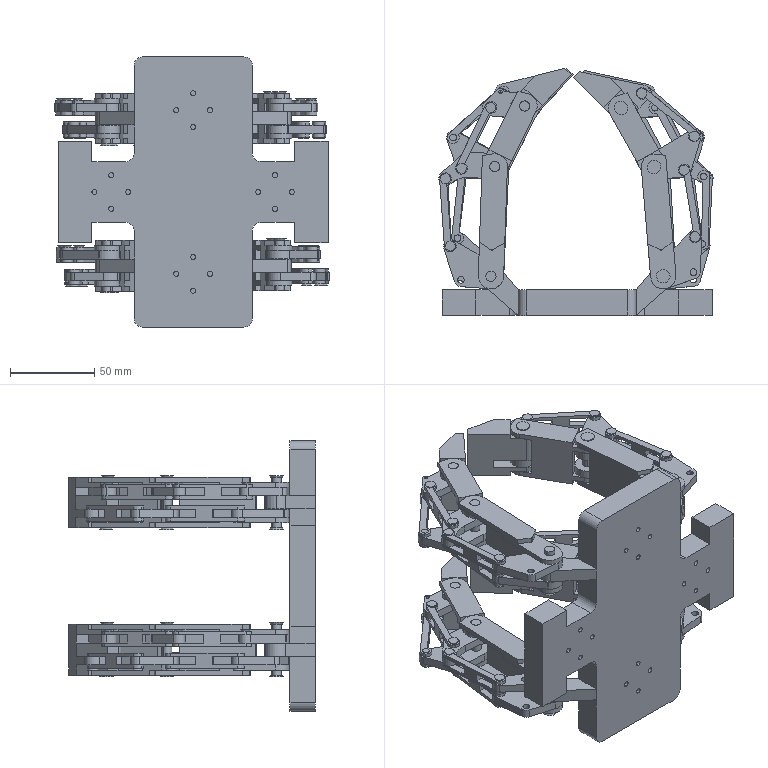Part | SolidWorks | 93 solids | 1500 faces | box 162.597 x 146.118 x 160 mm | volume 452731 mm3 | cylinder 722 | plane 690 | cone 88 | commonest cylinder face diameters 4 x276 6 x148 7 x96 15 x76 3 x32 10 x32